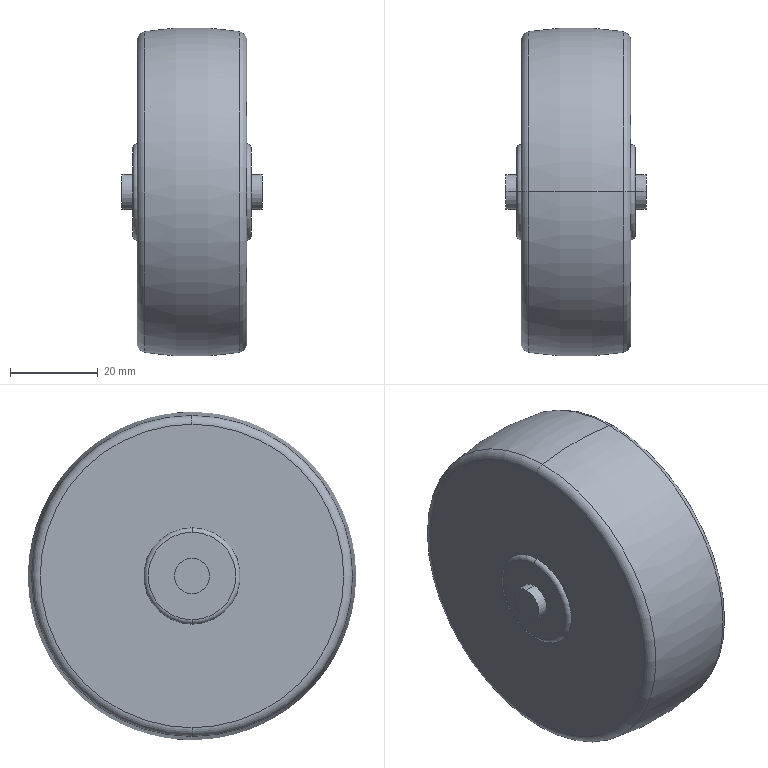Part | SolidWorks | features BaseBody 1 | 1 solid | 20 faces | box 32 x 75 x 75 mm | volume 108825 mm3 | torus 10 | plane 6 | cylinder 4 | commonest cylinder face diameters 8 x4
STEP:
#1=CARTESIAN_POINT('',(13.5,0.,-4.));
#2=VERTEX_POINT('',#1);
#3=CARTESIAN_POINT('',(13.5,0.,4.));
#4=VERTEX_POINT('',#3);
#5=CARTESIAN_POINT('',(13.5,0.,0.));
#6=DIRECTION('',(1.,0.,0.));
#7=DIRECTION('',(0.,0.,-1.));
#8=AXIS2_PLACEMENT_3D('',#5,#6,#7);
#9=CIRCLE('',#8,4.);
#10=EDGE_CURVE('',#2,#4,#9,.T.);
#11=ORIENTED_EDGE('',*,*,#10,.T.);
#12=CARTESIAN_POINT('',(16.,0.,4.));
#13=VERTEX_POINT('',#12);
#14=CARTESIAN_POINT('',(16.,0.,4.));
#15=DIRECTION('',(1.,0.,0.));
#16=VECTOR('',#15,1000.);
#17=LINE('',#14,#16);
#18=EDGE_CURVE('',#4,#13,#17,.T.);
#19=ORIENTED_EDGE('',*,*,#18,.T.);
#20=CARTESIAN_POINT('',(16.,0.,-4.));
#21=VERTEX_POINT('',#20);
#22=CARTESIAN_POINT('',(16.,0.,0.));
#23=DIRECTION('',(1.,0.,0.));
#24=DIRECTION('',(0.,0.,-1.));
#25=AXIS2_PLACEMENT_3D('',#22,#23,#24);
#26=CIRCLE('',#25,4.);
#27=EDGE_CURVE('',#21,#13,#26,.T.);
#28=ORIENTED_EDGE('',*,*,#27,.F.);
#29=CARTESIAN_POINT('',(16.,0.,-4.));
#30=DIRECTION('',(1.,0.,0.));
#31=VECTOR('',#30,1000.);
#32=LINE('',#29,#31);
#33=EDGE_CURVE('',#2,#21,#32,.T.);
#34=ORIENTED_EDGE('',*,*,#33,.F.);
#35=EDGE_LOOP('',(#11,#19,#28,#34));
#36=FACE_OUTER_BOUND('',#35,.T.);
#37=CARTESIAN_POINT('',(16.,0.,0.));
#38=DIRECTION('',(1.,0.,0.));
#39=DIRECTION('',(0.,0.,-1.));
#40=AXIS2_PLACEMENT_3D('',#37,#38,#39);
#41=CYLINDRICAL_SURFACE('',#40,4.);
#42=ADVANCED_FACE('',(#36),#41,.T.);
#43=CARTESIAN_POINT('',(12.5,0.,-11.));
#44=VERTEX_POINT('',#43);
#45=CARTESIAN_POINT('',(12.5,0.,11.));
#46=VERTEX_POINT('',#45);
#47=CARTESIAN_POINT('',(12.5,0.,0.));
#48=DIRECTION('',(1.,0.,0.));
#49=DIRECTION('',(0.,0.,-1.));
#50=AXIS2_PLACEMENT_3D('',#47,#48,#49);
#51=CIRCLE('',#50,11.);
#52=EDGE_CURVE('',#44,#46,#51,.T.);
#53=ORIENTED_EDGE('',*,*,#52,.T.);
#54=CARTESIAN_POINT('',(13.5,0.,10.));
#55=VERTEX_POINT('',#54);
#56=CARTESIAN_POINT('',(12.5,0.,10.));
#57=DIRECTION('',(0.,1.,0.));
#58=DIRECTION('',(0.,0.,1.));
#59=AXIS2_PLACEMENT_3D('',#56,#57,#58);
#60=CIRCLE('',#59,1.);
#61=EDGE_CURVE('',#46,#55,#60,.T.);
#62=ORIENTED_EDGE('',*,*,#61,.T.);
#63=CARTESIAN_POINT('',(13.5,0.,-10.));
#64=VERTEX_POINT('',#63);
#65=CARTESIAN_POINT('',(13.5,0.,0.));
#66=DIRECTION('',(1.,0.,0.));
#67=DIRECTION('',(0.,0.,-1.));
#68=AXIS2_PLACEMENT_3D('',#65,#66,#67);
#69=CIRCLE('',#68,10.);
#70=EDGE_CURVE('',#64,#55,#69,.T.);
#71=ORIENTED_EDGE('',*,*,#70,.F.);
#72=CARTESIAN_POINT('',(12.5,0.,-10.));
#73=DIRECTION('',(0.,-1.,0.));
#74=DIRECTION('',(0.,0.,-1.));
#75=AXIS2_PLACEMENT_3D('',#72,#73,#74);
#76=CIRCLE('',#75,1.);
#77=EDGE_CURVE('',#44,#64,#76,.T.);
#78=ORIENTED_EDGE('',*,*,#77,.F.);
#79=EDGE_LOOP('',(#53,#62,#71,#78));
#80=FACE_OUTER_BOUND('',#79,.T.);
#81=CARTESIAN_POINT('',(12.5,0.,0.));
#82=DIRECTION('',(1.,0.,0.));
#83=DIRECTION('',(0.,0.,-1.));
#84=AXIS2_PLACEMENT_3D('',#81,#82,#83);
#85=TOROIDAL_SURFACE('',#84,10.,1.);
#86=ADVANCED_FACE('',(#80),#85,.T.);
#87=CARTESIAN_POINT('',(10.833,0.,-36.591));
#88=VERTEX_POINT('',#87);
#89=CARTESIAN_POINT('',(10.833,0.,36.591));
#90=VERTEX_POINT('',#89);
#91=CARTESIAN_POINT('',(10.833,0.,0.));
#92=DIRECTION('',(1.,0.,0.));
#93=DIRECTION('',(0.,0.,-1.));
#94=AXIS2_PLACEMENT_3D('',#91,#92,#93);
#95=CIRCLE('',#94,36.591);
#96=EDGE_CURVE('',#88,#90,#95,.T.);
#97=ORIENTED_EDGE('',*,*,#96,.T.);
#98=CARTESIAN_POINT('',(12.5,0.,34.619));
#99=VERTEX_POINT('',#98);
#100=CARTESIAN_POINT('',(10.5,0.,34.619));
#101=DIRECTION('',(0.,1.,0.));
#102=DIRECTION('',(0.,0.,1.));
#103=AXIS2_PLACEMENT_3D('',#100,#101,#102);
#104=CIRCLE('',#103,2.);
#105=EDGE_CURVE('',#90,#99,#104,.T.);
#106=ORIENTED_EDGE('',*,*,#105,.T.);
#107=CARTESIAN_POINT('',(12.5,0.,-34.619));
#108=VERTEX_POINT('',#107);
#109=CARTESIAN_POINT('',(12.5,0.,0.));
#110=DIRECTION('',(1.,0.,0.));
#111=DIRECTION('',(0.,0.,-1.));
#112=AXIS2_PLACEMENT_3D('',#109,#110,#111);
#113=CIRCLE('',#112,34.619);
#114=EDGE_CURVE('',#108,#99,#113,.T.);
#115=ORIENTED_EDGE('',*,*,#114,.F.);
#116=CARTESIAN_POINT('',(10.5,0.,-34.619));
#117=DIRECTION('',(0.,-1.,0.));
#118=DIRECTION('',(0.,0.,-1.));
#119=AXIS2_PLACEMENT_3D('',#116,#117,#118);
#120=CIRCLE('',#119,2.);
#121=EDGE_CURVE('',#88,#108,#120,.T.);
#122=ORIENTED_EDGE('',*,*,#121,.F.);
#123=EDGE_LOOP('',(#97,#106,#115,#122));
#124=FACE_OUTER_BOUND('',#123,.T.);
#125=CARTESIAN_POINT('',(10.5,0.,0.));
#126=DIRECTION('',(1.,0.,0.));
#127=DIRECTION('',(0.,0.,-1.));
#128=AXIS2_PLACEMENT_3D('',#125,#126,#127);
#129=TOROIDAL_SURFACE('',#128,34.619,2.);
#130=ADVANCED_FACE('',(#124),#129,.T.);
#131=CARTESIAN_POINT('',(-10.833,0.,-36.591));
#132=VERTEX_POINT('',#131);
#133=CARTESIAN_POINT('',(-10.833,0.,36.591));
#134=VERTEX_POINT('',#133);
#135=CARTESIAN_POINT('',(-10.833,0.,0.));
#136=DIRECTION('',(1.,0.,0.));
#137=DIRECTION('',(0.,0.,-1.));
#138=AXIS2_PLACEMENT_3D('',#135,#136,#137);
#139=CIRCLE('',#138,36.591);
#140=EDGE_CURVE('',#132,#134,#139,.T.);
#141=ORIENTED_EDGE('',*,*,#140,.T.);
#142=CARTESIAN_POINT('',(0.,0.,-27.5));
#143=DIRECTION('',(0.,1.,0.));
#144=DIRECTION('',(0.,0.,1.));
#145=AXIS2_PLACEMENT_3D('',#142,#143,#144);
#146=CIRCLE('',#145,65.);
#147=EDGE_CURVE('',#134,#90,#146,.T.);
#148=ORIENTED_EDGE('',*,*,#147,.T.);
#149=ORIENTED_EDGE('',*,*,#96,.F.);
#150=CARTESIAN_POINT('',(0.,0.,27.5));
#151=DIRECTION('',(0.,-1.,0.));
#152=DIRECTION('',(0.,0.,-1.));
#153=AXIS2_PLACEMENT_3D('',#150,#151,#152);
#154=CIRCLE('',#153,65.);
#155=EDGE_CURVE('',#132,#88,#154,.T.);
#156=ORIENTED_EDGE('',*,*,#155,.F.);
#157=EDGE_LOOP('',(#141,#148,#149,#156));
#158=FACE_OUTER_BOUND('',#157,.T.);
#159=CARTESIAN_POINT('',(0.,0.,0.));
#160=DIRECTION('',(1.,0.,0.));
#161=DIRECTION('',(0.,0.,-1.));
#162=AXIS2_PLACEMENT_3D('',#159,#160,#161);
#163=TOROIDAL_SURFACE('',#162,-27.5,65.);
#164=ADVANCED_FACE('',(#158),#163,.T.);
#165=CARTESIAN_POINT('',(-12.5,0.,-34.619));
#166=VERTEX_POINT('',#165);
#167=CARTESIAN_POINT('',(-12.5,0.,34.619));
#168=VERTEX_POINT('',#167);
#169=CARTESIAN_POINT('',(-12.5,0.,0.));
#170=DIRECTION('',(1.,0.,0.));
#171=DIRECTION('',(0.,0.,-1.));
#172=AXIS2_PLACEMENT_3D('',#169,#170,#171);
#173=CIRCLE('',#172,34.619);
#174=EDGE_CURVE('',#166,#168,#173,.T.);
#175=ORIENTED_EDGE('',*,*,#174,.T.);
#176=CARTESIAN_POINT('',(-10.5,0.,34.619));
#177=DIRECTION('',(0.,1.,0.));
#178=DIRECTION('',(0.,0.,1.));
#179=AXIS2_PLACEMENT_3D('',#176,#177,#178);
#180=CIRCLE('',#179,2.);
#181=EDGE_CURVE('',#168,#134,#180,.T.);
#182=ORIENTED_EDGE('',*,*,#181,.T.);
#183=ORIENTED_EDGE('',*,*,#140,.F.);
#184=CARTESIAN_POINT('',(-10.5,0.,-34.619));
#185=DIRECTION('',(0.,-1.,0.));
#186=DIRECTION('',(0.,0.,-1.));
#187=AXIS2_PLACEMENT_3D('',#184,#185,#186);
#188=CIRCLE('',#187,2.);
#189=EDGE_CURVE('',#166,#132,#188,.T.);
#190=ORIENTED_EDGE('',*,*,#189,.F.);
#191=EDGE_LOOP('',(#175,#182,#183,#190));
#192=FACE_OUTER_BOUND('',#191,.T.);
#193=CARTESIAN_POINT('',(-10.5,0.,0.));
#194=DIRECTION('',(1.,0.,0.));
#195=DIRECTION('',(0.,0.,-1.));
#196=AXIS2_PLACEMENT_3D('',#193,#194,#195);
#197=TOROIDAL_SURFACE('',#196,34.619,2.);
#198=ADVANCED_FACE('',(#192),#197,.T.);
#199=CARTESIAN_POINT('',(-13.5,0.,-10.));
#200=VERTEX_POINT('',#199);
#201=CARTESIAN_POINT('',(-13.5,0.,10.));
#202=VERTEX_POINT('',#201);
#203=CARTESIAN_POINT('',(-13.5,0.,0.));
#204=DIRECTION('',(1.,0.,0.));
#205=DIRECTION('',(0.,0.,-1.));
#206=AXIS2_PLACEMENT_3D('',#203,#204,#205);
#207=CIRCLE('',#206,10.);
#208=EDGE_CURVE('',#200,#202,#207,.T.);
#209=ORIENTED_EDGE('',*,*,#208,.T.);
#210=CARTESIAN_POINT('',(-12.5,0.,11.));
#211=VERTEX_POINT('',#210);
#212=CARTESIAN_POINT('',(-12.5,0.,10.));
#213=DIRECTION('',(0.,1.,0.));
#214=DIRECTION('',(0.,0.,1.));
#215=AXIS2_PLACEMENT_3D('',#212,#213,#214);
#216=CIRCLE('',#215,1.);
#217=EDGE_CURVE('',#202,#211,#216,.T.);
#218=ORIENTED_EDGE('',*,*,#217,.T.);
#219=CARTESIAN_POINT('',(-12.5,0.,-11.));
#220=VERTEX_POINT('',#219);
#221=CARTESIAN_POINT('',(-12.5,0.,0.));
#222=DIRECTION('',(1.,0.,0.));
#223=DIRECTION('',(0.,0.,-1.));
#224=AXIS2_PLACEMENT_3D('',#221,#222,#223);
#225=CIRCLE('',#224,11.);
#226=EDGE_CURVE('',#220,#211,#225,.T.);
#227=ORIENTED_EDGE('',*,*,#226,.F.);
#228=CARTESIAN_POINT('',(-12.5,0.,-10.));
#229=DIRECTION('',(0.,-1.,0.));
#230=DIRECTION('',(0.,0.,-1.));
#231=AXIS2_PLACEMENT_3D('',#228,#229,#230);
#232=CIRCLE('',#231,1.);
#233=EDGE_CURVE('',#200,#220,#232,.T.);
#234=ORIENTED_EDGE('',*,*,#233,.F.);
#235=EDGE_LOOP('',(#209,#218,#227,#234));
#236=FACE_OUTER_BOUND('',#235,.T.);
#237=CARTESIAN_POINT('',(-12.5,0.,0.));
#238=DIRECTION('',(1.,0.,0.));
#239=DIRECTION('',(0.,0.,-1.));
#240=AXIS2_PLACEMENT_3D('',#237,#238,#239);
#241=TOROIDAL_SURFACE('',#240,10.,1.);
#242=ADVANCED_FACE('',(#236),#241,.T.);
#243=CARTESIAN_POINT('',(-16.,0.,-4.));
#244=VERTEX_POINT('',#243);
#245=CARTESIAN_POINT('',(-16.,0.,4.));
#246=VERTEX_POINT('',#245);
#247=CARTESIAN_POINT('',(-16.,0.,0.));
#248=DIRECTION('',(1.,0.,0.));
#249=DIRECTION('',(0.,0.,-1.));
#250=AXIS2_PLACEMENT_3D('',#247,#248,#249);
#251=CIRCLE('',#250,4.);
#252=EDGE_CURVE('',#244,#246,#251,.T.);
#253=ORIENTED_EDGE('',*,*,#252,.T.);
#254=CARTESIAN_POINT('',(-13.5,0.,4.));
#255=VERTEX_POINT('',#254);
#256=CARTESIAN_POINT('',(16.,0.,4.));
#257=DIRECTION('',(1.,0.,0.));
#258=VECTOR('',#257,1000.);
#259=LINE('',#256,#258);
#260=EDGE_CURVE('',#246,#255,#259,.T.);
#261=ORIENTED_EDGE('',*,*,#260,.T.);
#262=CARTESIAN_POINT('',(-13.5,0.,-4.));
#263=VERTEX_POINT('',#262);
#264=CARTESIAN_POINT('',(-13.5,0.,0.));
#265=DIRECTION('',(1.,0.,0.));
#266=DIRECTION('',(0.,0.,-1.));
#267=AXIS2_PLACEMENT_3D('',#264,#265,#266);
#268=CIRCLE('',#267,4.);
#269=EDGE_CURVE('',#263,#255,#268,.T.);
#270=ORIENTED_EDGE('',*,*,#269,.F.);
#271=CARTESIAN_POINT('',(16.,0.,-4.));
#272=DIRECTION('',(1.,0.,0.));
#273=VECTOR('',#272,1000.);
#274=LINE('',#271,#273);
#275=EDGE_CURVE('',#244,#263,#274,.T.);
#276=ORIENTED_EDGE('',*,*,#275,.F.);
#277=EDGE_LOOP('',(#253,#261,#270,#276));
#278=FACE_OUTER_BOUND('',#277,.T.);
#279=CARTESIAN_POINT('',(16.,0.,0.));
#280=DIRECTION('',(1.,0.,0.));
#281=DIRECTION('',(0.,0.,-1.));
#282=AXIS2_PLACEMENT_3D('',#279,#280,#281);
#283=CYLINDRICAL_SURFACE('',#282,4.);
#284=ADVANCED_FACE('',(#278),#283,.T.);
#285=ORIENTED_EDGE('',*,*,#252,.F.);
#286=CARTESIAN_POINT('',(-16.,0.,0.));
#287=DIRECTION('',(1.,0.,0.));
#288=DIRECTION('',(0.,0.,-1.));
#289=AXIS2_PLACEMENT_3D('',#286,#287,#288);
#290=CIRCLE('',#289,4.);
#291=EDGE_CURVE('',#246,#244,#290,.T.);
#292=ORIENTED_EDGE('',*,*,#291,.F.);
#293=EDGE_LOOP('',(#285,#292));
#294=FACE_OUTER_BOUND('',#293,.T.);
#295=CARTESIAN_POINT('',(-16.,0.,0.));
#296=DIRECTION('',(1.,0.,0.));
#297=DIRECTION('',(0.,0.,-1.));
#298=AXIS2_PLACEMENT_3D('',#295,#296,#297);
#299=PLANE('',#298);
#300=ADVANCED_FACE('',(#294),#299,.F.);
#301=ORIENTED_EDGE('',*,*,#260,.F.);
#302=ORIENTED_EDGE('',*,*,#291,.T.);
#303=ORIENTED_EDGE('',*,*,#275,.T.);
#304=CARTESIAN_POINT('',(-13.5,0.,0.));
#305=DIRECTION('',(1.,0.,0.));
#306=DIRECTION('',(0.,0.,-1.));
#307=AXIS2_PLACEMENT_3D('',#304,#305,#306);
#308=CIRCLE('',#307,4.);
#309=EDGE_CURVE('',#255,#263,#308,.T.);
#310=ORIENTED_EDGE('',*,*,#309,.F.);
#311=EDGE_LOOP('',(#301,#302,#303,#310));
#312=FACE_OUTER_BOUND('',#311,.T.);
#313=CARTESIAN_POINT('',(16.,0.,0.));
#314=DIRECTION('',(1.,0.,0.));
#315=DIRECTION('',(0.,0.,-1.));
#316=AXIS2_PLACEMENT_3D('',#313,#314,#315);
#317=CYLINDRICAL_SURFACE('',#316,4.);
#318=ADVANCED_FACE('',(#312),#317,.T.);
#319=ORIENTED_EDGE('',*,*,#208,.F.);
#320=CARTESIAN_POINT('',(-13.5,0.,0.));
#321=DIRECTION('',(1.,0.,0.));
#322=DIRECTION('',(0.,0.,-1.));
#323=AXIS2_PLACEMENT_3D('',#320,#321,#322);
#324=CIRCLE('',#323,10.);
#325=EDGE_CURVE('',#202,#200,#324,.T.);
#326=ORIENTED_EDGE('',*,*,#325,.F.);
#327=EDGE_LOOP('',(#319,#326));
#328=FACE_OUTER_BOUND('',#327,.T.);
#329=ORIENTED_EDGE('',*,*,#269,.T.);
#330=ORIENTED_EDGE('',*,*,#309,.T.);
#331=EDGE_LOOP('',(#329,#330));
#332=FACE_BOUND('',#331,.T.);
#333=CARTESIAN_POINT('',(-13.5,4.,0.));
#334=DIRECTION('',(1.,0.,0.));
#335=DIRECTION('',(0.,0.,-1.));
#336=AXIS2_PLACEMENT_3D('',#333,#334,#335);
#337=PLANE('',#336);
#338=ADVANCED_FACE('',(#328,#332),#337,.F.);
#339=ORIENTED_EDGE('',*,*,#217,.F.);
#340=ORIENTED_EDGE('',*,*,#325,.T.);
#341=ORIENTED_EDGE('',*,*,#233,.T.);
#342=CARTESIAN_POINT('',(-12.5,0.,0.));
#343=DIRECTION('',(1.,0.,0.));
#344=DIRECTION('',(0.,0.,-1.));
#345=AXIS2_PLACEMENT_3D('',#342,#343,#344);
#346=CIRCLE('',#345,11.);
#347=EDGE_CURVE('',#211,#220,#346,.T.);
#348=ORIENTED_EDGE('',*,*,#347,.F.);
#349=EDGE_LOOP('',(#339,#340,#341,#348));
#350=FACE_OUTER_BOUND('',#349,.T.);
#351=CARTESIAN_POINT('',(-12.5,0.,0.));
#352=DIRECTION('',(1.,0.,0.));
#353=DIRECTION('',(0.,0.,-1.));
#354=AXIS2_PLACEMENT_3D('',#351,#352,#353);
#355=TOROIDAL_SURFACE('',#354,10.,1.);
#356=ADVANCED_FACE('',(#350),#355,.T.);
#357=ORIENTED_EDGE('',*,*,#174,.F.);
#358=CARTESIAN_POINT('',(-12.5,0.,0.));
#359=DIRECTION('',(1.,0.,0.));
#360=DIRECTION('',(0.,0.,-1.));
#361=AXIS2_PLACEMENT_3D('',#358,#359,#360);
#362=CIRCLE('',#361,34.619);
#363=EDGE_CURVE('',#168,#166,#362,.T.);
#364=ORIENTED_EDGE('',*,*,#363,.F.);
#365=EDGE_LOOP('',(#357,#364));
#366=FACE_OUTER_BOUND('',#365,.T.);
#367=ORIENTED_EDGE('',*,*,#226,.T.);
#368=ORIENTED_EDGE('',*,*,#347,.T.);
#369=EDGE_LOOP('',(#367,#368));
#370=FACE_BOUND('',#369,.T.);
#371=CARTESIAN_POINT('',(-12.5,11.,0.));
#372=DIRECTION('',(1.,0.,0.));
#373=DIRECTION('',(0.,0.,-1.));
#374=AXIS2_PLACEMENT_3D('',#371,#372,#373);
#375=PLANE('',#374);
#376=ADVANCED_FACE('',(#366,#370),#375,.F.);
#377=ORIENTED_EDGE('',*,*,#181,.F.);
#378=ORIENTED_EDGE('',*,*,#363,.T.);
#379=ORIENTED_EDGE('',*,*,#189,.T.);
#380=CARTESIAN_POINT('',(-10.833,0.,0.));
#381=DIRECTION('',(1.,0.,0.));
#382=DIRECTION('',(0.,0.,-1.));
#383=AXIS2_PLACEMENT_3D('',#380,#381,#382);
#384=CIRCLE('',#383,36.591);
#385=EDGE_CURVE('',#134,#132,#384,.T.);
#386=ORIENTED_EDGE('',*,*,#385,.F.);
#387=EDGE_LOOP('',(#377,#378,#379,#386));
#388=FACE_OUTER_BOUND('',#387,.T.);
#389=CARTESIAN_POINT('',(-10.5,0.,0.));
#390=DIRECTION('',(1.,0.,0.));
#391=DIRECTION('',(0.,0.,-1.));
#392=AXIS2_PLACEMENT_3D('',#389,#390,#391);
#393=TOROIDAL_SURFACE('',#392,34.619,2.);
#394=ADVANCED_FACE('',(#388),#393,.T.);
#395=ORIENTED_EDGE('',*,*,#147,.F.);
#396=ORIENTED_EDGE('',*,*,#385,.T.);
#397=ORIENTED_EDGE('',*,*,#155,.T.);
#398=CARTESIAN_POINT('',(10.833,0.,0.));
#399=DIRECTION('',(1.,0.,0.));
#400=DIRECTION('',(0.,0.,-1.));
#401=AXIS2_PLACEMENT_3D('',#398,#399,#400);
#402=CIRCLE('',#401,36.591);
#403=EDGE_CURVE('',#90,#88,#402,.T.);
#404=ORIENTED_EDGE('',*,*,#403,.F.);
#405=EDGE_LOOP('',(#395,#396,#397,#404));
#406=FACE_OUTER_BOUND('',#405,.T.);
#407=CARTESIAN_POINT('',(0.,0.,0.));
#408=DIRECTION('',(1.,0.,0.));
#409=DIRECTION('',(0.,0.,-1.));
#410=AXIS2_PLACEMENT_3D('',#407,#408,#409);
#411=TOROIDAL_SURFACE('',#410,-27.5,65.);
#412=ADVANCED_FACE('',(#406),#411,.T.);
#413=ORIENTED_EDGE('',*,*,#105,.F.);
#414=ORIENTED_EDGE('',*,*,#403,.T.);
#415=ORIENTED_EDGE('',*,*,#121,.T.);
#416=CARTESIAN_POINT('',(12.5,0.,0.));
#417=DIRECTION('',(1.,0.,0.));
#418=DIRECTION('',(0.,0.,-1.));
#419=AXIS2_PLACEMENT_3D('',#416,#417,#418);
#420=CIRCLE('',#419,34.619);
#421=EDGE_CURVE('',#99,#108,#420,.T.);
#422=ORIENTED_EDGE('',*,*,#421,.F.);
#423=EDGE_LOOP('',(#413,#414,#415,#422));
#424=FACE_OUTER_BOUND('',#423,.T.);
#425=CARTESIAN_POINT('',(10.5,0.,0.));
#426=DIRECTION('',(1.,0.,0.));
#427=DIRECTION('',(0.,0.,-1.));
#428=AXIS2_PLACEMENT_3D('',#425,#426,#427);
#429=TOROIDAL_SURFACE('',#428,34.619,2.);
#430=ADVANCED_FACE('',(#424),#429,.T.);
#431=ORIENTED_EDGE('',*,*,#52,.F.);
#432=CARTESIAN_POINT('',(12.5,0.,0.));
#433=DIRECTION('',(1.,0.,0.));
#434=DIRECTION('',(0.,0.,-1.));
#435=AXIS2_PLACEMENT_3D('',#432,#433,#434);
#436=CIRCLE('',#435,11.);
#437=EDGE_CURVE('',#46,#44,#436,.T.);
#438=ORIENTED_EDGE('',*,*,#437,.F.);
#439=EDGE_LOOP('',(#431,#438));
#440=FACE_BOUND('',#439,.T.);
#441=ORIENTED_EDGE('',*,*,#114,.T.);
#442=ORIENTED_EDGE('',*,*,#421,.T.);
#443=EDGE_LOOP('',(#441,#442));
#444=FACE_OUTER_BOUND('',#443,.T.);
#445=CARTESIAN_POINT('',(12.5,34.619,0.));
#446=DIRECTION('',(-1.,0.,0.));
#447=DIRECTION('',(0.,0.,1.));
#448=AXIS2_PLACEMENT_3D('',#445,#446,#447);
#449=PLANE('',#448);
#450=ADVANCED_FACE('',(#440,#444),#449,.F.);
#451=ORIENTED_EDGE('',*,*,#61,.F.);
#452=ORIENTED_EDGE('',*,*,#437,.T.);
#453=ORIENTED_EDGE('',*,*,#77,.T.);
#454=CARTESIAN_POINT('',(13.5,0.,0.));
#455=DIRECTION('',(1.,0.,0.));
#456=DIRECTION('',(0.,0.,-1.));
#457=AXIS2_PLACEMENT_3D('',#454,#455,#456);
#458=CIRCLE('',#457,10.);
#459=EDGE_CURVE('',#55,#64,#458,.T.);
#460=ORIENTED_EDGE('',*,*,#459,.F.);
#461=EDGE_LOOP('',(#451,#452,#453,#460));
#462=FACE_OUTER_BOUND('',#461,.T.);
#463=CARTESIAN_POINT('',(12.5,0.,0.));
#464=DIRECTION('',(1.,0.,0.));
#465=DIRECTION('',(0.,0.,-1.));
#466=AXIS2_PLACEMENT_3D('',#463,#464,#465);
#467=TOROIDAL_SURFACE('',#466,10.,1.);
#468=ADVANCED_FACE('',(#462),#467,.T.);
#469=ORIENTED_EDGE('',*,*,#10,.F.);
#470=CARTESIAN_POINT('',(13.5,0.,0.));
#471=DIRECTION('',(1.,0.,0.));
#472=DIRECTION('',(0.,0.,-1.));
#473=AXIS2_PLACEMENT_3D('',#470,#471,#472);
#474=CIRCLE('',#473,4.);
#475=EDGE_CURVE('',#4,#2,#474,.T.);
#476=ORIENTED_EDGE('',*,*,#475,.F.);
#477=EDGE_LOOP('',(#469,#476));
#478=FACE_BOUND('',#477,.T.);
#479=ORIENTED_EDGE('',*,*,#70,.T.);
#480=ORIENTED_EDGE('',*,*,#459,.T.);
#481=EDGE_LOOP('',(#479,#480));
#482=FACE_OUTER_BOUND('',#481,.T.);
#483=CARTESIAN_POINT('',(13.5,10.,0.));
#484=DIRECTION('',(-1.,0.,0.));
#485=DIRECTION('',(0.,0.,1.));
#486=AXIS2_PLACEMENT_3D('',#483,#484,#485);
#487=PLANE('',#486);
#488=ADVANCED_FACE('',(#478,#482),#487,.F.);
#489=ORIENTED_EDGE('',*,*,#18,.F.);
#490=ORIENTED_EDGE('',*,*,#475,.T.);
#491=ORIENTED_EDGE('',*,*,#33,.T.);
#492=CARTESIAN_POINT('',(16.,0.,0.));
#493=DIRECTION('',(1.,0.,0.));
#494=DIRECTION('',(0.,0.,-1.));
#495=AXIS2_PLACEMENT_3D('',#492,#493,#494);
#496=CIRCLE('',#495,4.);
#497=EDGE_CURVE('',#13,#21,#496,.T.);
#498=ORIENTED_EDGE('',*,*,#497,.F.);
#499=EDGE_LOOP('',(#489,#490,#491,#498));
#500=FACE_OUTER_BOUND('',#499,.T.);
#501=CARTESIAN_POINT('',(16.,0.,0.));
#502=DIRECTION('',(1.,0.,0.));
#503=DIRECTION('',(0.,0.,-1.));
#504=AXIS2_PLACEMENT_3D('',#501,#502,#503);
#505=CYLINDRICAL_SURFACE('',#504,4.);
#506=ADVANCED_FACE('',(#500),#505,.T.);
#507=ORIENTED_EDGE('',*,*,#27,.T.);
#508=ORIENTED_EDGE('',*,*,#497,.T.);
#509=EDGE_LOOP('',(#507,#508));
#510=FACE_OUTER_BOUND('',#509,.T.);
#511=CARTESIAN_POINT('',(16.,4.,0.));
#512=DIRECTION('',(-1.,0.,0.));
#513=DIRECTION('',(0.,0.,1.));
#514=AXIS2_PLACEMENT_3D('',#511,#512,#513);
#515=PLANE('',#514);
#516=ADVANCED_FACE('',(#510),#515,.F.);
#517=CLOSED_SHELL('',(#42,#86,#130,#164,#198,#242,#284,#300,#318,#338,#356,#376,#394,#412,#430,#450,#468,#488,#506,#516));
#518=MANIFOLD_SOLID_BREP('',#517);
#519=CARTESIAN_POINT('',(0.,0.,0.));
#520=DIRECTION('',(0.,0.,1.));
#521=DIRECTION('',(1.,0.,0.));
#522=AXIS2_PLACEMENT_3D('',#519,#520,#521);
#523=(LENGTH_UNIT()NAMED_UNIT(*)SI_UNIT(.MILLI.,.METRE.));
#524=UNCERTAINTY_MEASURE_WITH_UNIT(LENGTH_MEASURE(0.00001),#523,'','');
#525=(NAMED_UNIT(*)PLANE_ANGLE_UNIT()SI_UNIT($,.RADIAN.));
#526=(NAMED_UNIT(*)SI_UNIT($,.STERADIAN.)SOLID_ANGLE_UNIT());
#527=(GEOMETRIC_REPRESENTATION_CONTEXT(3)GLOBAL_UNCERTAINTY_ASSIGNED_CONTEXT((#524))GLOBAL_UNIT_ASSIGNED_CONTEXT((#523,#525,#526))REPRESENTATION_CONTEXT('',''));
#528=ADVANCED_BREP_SHAPE_REPRESENTATION('',(#518,#522),#527);